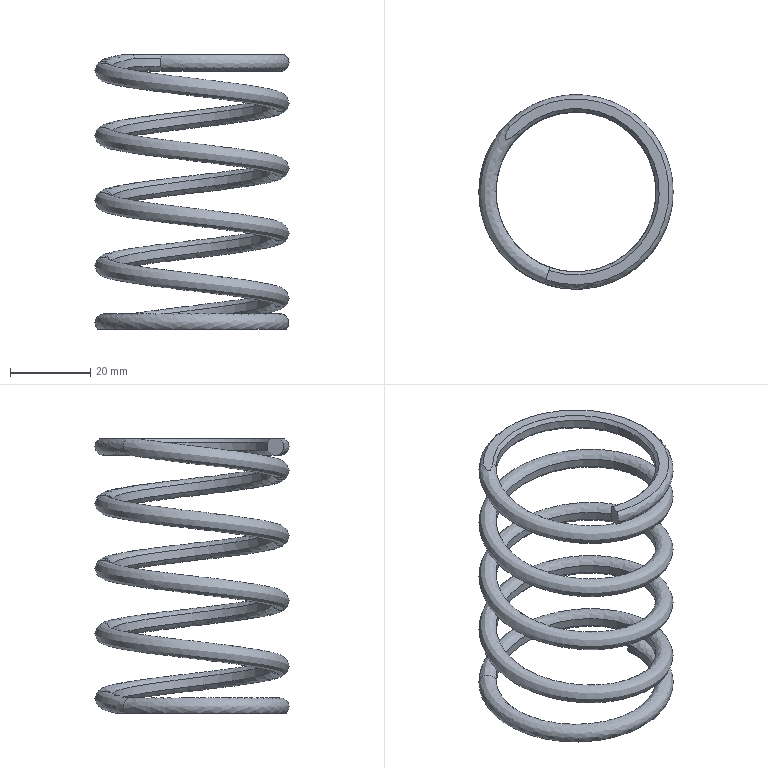Part | STEP file | PN_0006_default | 1 solid | 10 faces | volume 11391 mm3 | spline 5 | plane 4 | cylinder 1 | commonest cylinder face diameters 40 x1